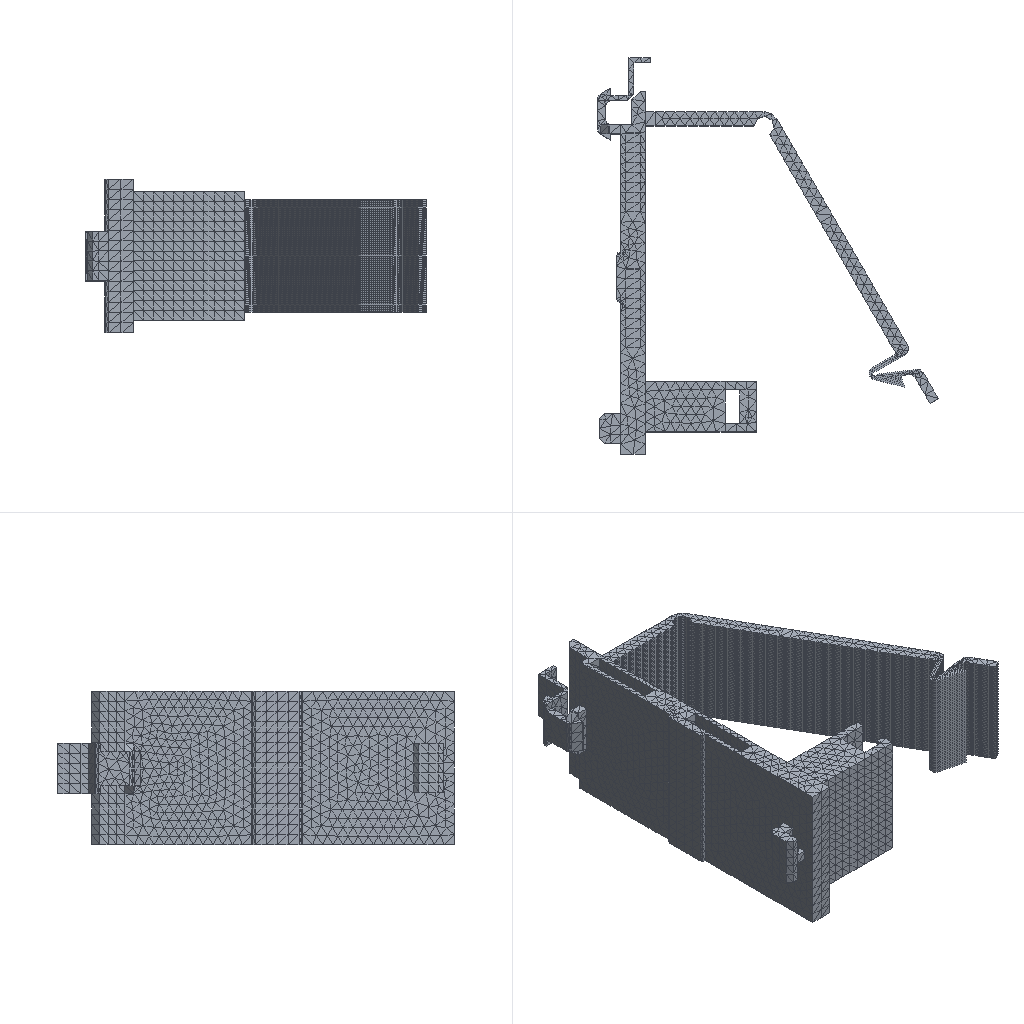Simulation study | abaqus
Set-up summary:
category,name,step,type,value,unit,region
solver,abaqus
solver,version,,,Abaqus/Standard 2020
units,not stated in the deck,,not stated
analysis,deck,,static,static
load_step,Step-1,Step-1,static
load_step,requested,,,1
mesh,nodes,,,22075
mesh,elements,,,90547
element_type,C3D4,,solid,90547
load,load commands in deck,,count,1
bc,support commands in deck,,count,7
material,MATERIAL-1,,in results
check,setup vs results,,match,"per instance, exact: element labels, types and connectivity; labels of the nodes the elements use; coordinates of those nodes at SINGLE_PRECISION in 1 of 1 instance(s)"
Abaqus input file, long lists of numbers shortened:
*Heading
** Job name: Job-2 Model name: Model-1
** Generated by: Abaqus/CAE 2020
*Preprint, echo=NO, model=NO, history=NO, contact=NO
**
** PARTS
**
*Part, name=work
*Node
      1,   3.807,  -1.262,   3.7
      2,   3.807,  -1.262,  -1.3
** (22073 more lines like these left out)
*Element, type=C3D4
    1, 14591, 14592, 14593, 14594
    2, 14591, 14595, 14596, 14594
** (90545 more lines like these left out)
*Nset, nset=Set-1, generate
     1,  22075,      1
*Elset, elset=Set-1, generate
     1,  90547,      1
** Section: Section-1
*Solid Section, elset=Set-1, material=Material-1
,
*End Part
**
**
** ASSEMBLY
**
*Assembly, name=Assembly
**
*Instance, name=work-1, part=work
*End Instance
**
*Node
      1,   16.658,   -4.462,         1.25
*Nset, nset=Set-3, instance=work-1
   104,   105,   106,   107,   108,   109,   110,   111,   112,   113,   114,   115,   116,   117,   118,   119
   120,   121,   122,   123,   205,   206,   209,   210,   217,   218,   219,   220,   223,   224,   225,   226
** (39 more lines like these left out)
*Elset, elset=Set-3, instance=work-1
   764,  2513,  4548,  6615,  8547,  8655,  9392,  9664, 10545, 10554, 10556, 10558, 10654, 10686, 12815, 12833
 12986, 12996, 13206, 13221, 13236, 13284, 13291, 13305, 13322, 13328, 13394, 13404, 13464, 13696, 14142, 15031
** (67 more lines like these left out)
*Nset, nset=Set-5
 1,
*Nset, nset=Set-6
 1,
*Nset, nset=m_Set-4
 1,
*Elset, elset=_s_Surf-1_S3, internal, instance=work-1
  1065,  3300,  9440,  9995, 12958, 13079, 13080, 13460, 13489, 13508, 13525, 13528, 13554, 13560, 13588, 13594
 14445, 14569, 14627, 14642, 14709, 14762, 14820, 15162, 15602, 15804, 16461, 17184, 17417, 17502, 18000, 18113
** (25 more lines like these left out)
*Elset, elset=_s_Surf-1_S4, internal, instance=work-1
  6947, 12110, 15494, 16739, 18273, 18904, 19107, 19441, 19514, 19558, 19605, 19740, 19774, 19808, 19878, 19909
 20085, 20116, 20253, 20968, 22709, 22964, 23125, 23432, 23584, 23605, 23741, 23742, 24158, 27091, 28853, 29818
** (2 more lines like these left out)
*Elset, elset=_s_Surf-1_S2, internal, instance=work-1
 13451, 18900, 19170, 19176, 19242, 19571, 19647, 19726, 19743, 19765, 19805, 19862, 19891, 20231, 20471, 20554
 21449, 23038, 23278, 23984, 23988, 29549, 29842, 30438, 33077, 33421, 39209, 54948, 58478, 69951, 70831, 76509
** (1 more lines like these left out)
*Elset, elset=_s_Surf-1_S1, internal, instance=work-1
 19134, 19251, 19392, 19742, 19751, 19762, 19798, 19846, 20167, 20178, 21353, 21370, 21694, 21764, 22003, 22004
 22470, 22799, 23500, 24551, 57766, 58494, 65889, 68364, 70026, 70454
*Surface, type=ELEMENT, name=s_Surf-1
_s_Surf-1_S3, S3
_s_Surf-1_S4, S4
_s_Surf-1_S2, S2
_s_Surf-1_S1, S1
*Elset, elset=_s_Surf-2_S4, internal, instance=work-1
  1164,  2199,  2690,  2870,  5811,  7944,  8257, 14253, 15244, 15617, 18853, 18854, 18866, 19575, 20898, 22227
 25708, 26415, 26669, 30098, 34360, 34378, 34963, 38395, 39354, 39389, 39423, 40444, 44348, 49840, 49921, 49978
** (5 more lines like these left out)
*Elset, elset=_s_Surf-2_S3, internal, instance=work-1
  6874, 12126, 12932, 13529, 14256, 14836, 15100, 15487, 15540, 15634, 16632, 17397, 18548, 18641, 18714, 18830
 19147, 19183, 19598, 19628, 19654, 19686, 19737, 19806, 19872, 19880, 20125, 21047, 21733, 21860, 22063, 22346
** (10 more lines like these left out)
*Elset, elset=_s_Surf-2_S1, internal, instance=work-1
 14248, 21140, 23265, 52910, 55080, 56694, 58541, 63758, 66566, 66615, 76146, 78774, 81565
*Elset, elset=_s_Surf-2_S2, internal, instance=work-1
 14684, 14796, 14845, 18949, 21197, 23723, 46722, 49241, 53451, 53829, 53860, 54862, 57325, 58957, 59065, 59920
 64158, 64175, 64252, 64405, 64463, 65348, 66297, 66598, 66650, 66991, 67034
*Surface, type=ELEMENT, name=s_Surf-2
_s_Surf-2_S4, S4
_s_Surf-2_S3, S3
_s_Surf-2_S2, S2
_s_Surf-2_S1, S1
*Elset, elset=_s_Surf-3_S4, internal, instance=work-1
   404,  1164,  1394,  1967,  2199,  2622,  2690,  2870,  3029,  3371,  3477,  3657,  5811,  6405,  6676,  7454
  7944,  8257, 11476, 14018, 14253, 14320, 15244, 15617, 17242, 18853, 18854, 18866, 18868, 19575, 19757, 20697
** (16 more lines like these left out)
*Elset, elset=_s_Surf-3_S3, internal, instance=work-1
   328,  1284,  2264,  2933,  3915,  6874,  7452,  7511,  9238, 11335, 11469, 11477, 11770, 12126, 12171, 12790
 12932, 12950, 12960, 12970, 13019, 13023, 13024, 13041, 13193, 13198, 13529, 13699, 13811, 13904, 13908, 13926
** (171 more lines like these left out)
*Elset, elset=_s_Surf-3_S1, internal, instance=work-1
   402,  2739,  4954,  6226, 11472, 12294, 14248, 15462, 20277, 20593, 21140, 23265, 24220, 29011, 29138, 29591
 30557, 30652, 30849, 31337, 31404, 31694, 33257, 33859, 34476, 34520, 34624, 34676, 34723, 34739, 35469, 35855
** (4 more lines like these left out)
*Elset, elset=_s_Surf-3_S2, internal, instance=work-1
  1620,  2009,  2935,  6231, 14684, 14796, 14845, 17188, 18949, 21197, 23723, 24383, 30551, 31366, 31614, 35305
 37994, 39980, 39981, 39988, 40055, 40547, 41770, 42297, 42310, 42420, 42471, 42925, 43365, 43770, 44062, 44070
** (3 more lines like these left out)
*Surface, type=ELEMENT, name=s_Surf-3
_s_Surf-3_S4, S4
_s_Surf-3_S3, S3
_s_Surf-3_S2, S2
_s_Surf-3_S1, S1
*Elset, elset=_s_Surf-4_S3, internal, instance=work-1
   328,  1284,  2264,  2933,  3915,  7452,  7511,  9238, 11335, 11469, 11477, 11770, 12171, 12790, 12950, 12960
 12970, 13019, 13023, 13024, 13041, 13193, 13198, 13699, 13811, 13904, 13908, 13926, 13943, 13948, 13953, 13961
** (159 more lines like these left out)
*Elset, elset=_s_Surf-4_S1, internal, instance=work-1
   402,  2739,  4954,  6226, 11472, 12294, 15462, 20277, 20593, 24220, 29011, 29138, 29591, 30557, 30652, 30849
 31337, 31404, 31694, 33257, 33859, 34476, 34520, 34624, 34676, 34723, 34739, 35469, 35855, 36039, 36429, 36634
** (3 more lines like these left out)
*Elset, elset=_s_Surf-4_S4, internal, instance=work-1
   404,  1394,  1967,  2622,  3029,  3371,  3477,  3657,  6405,  6676,  7454, 11476, 14018, 14320, 17242, 18868
 19757, 20697, 21384, 22882, 27591, 28591, 28728, 29631, 30272, 31136, 31264, 32150, 32937, 33001, 33241, 33489
** (9 more lines like these left out)
*Elset, elset=_s_Surf-4_S2, internal, instance=work-1
  1620,  2009,  2935,  6231, 17188, 24383, 30551, 31366, 31614, 35305, 37994, 39980, 39981, 39988, 40055, 40547
 41770, 42297, 42310, 42420, 42471, 42925, 43365, 43770, 44062, 44070, 44524, 46633, 47644, 47824, 48131, 59119
** (1 more lines like these left out)
*Surface, type=ELEMENT, name=s_Surf-4
_s_Surf-4_S3, S3
_s_Surf-4_S1, S1
_s_Surf-4_S4, S4
_s_Surf-4_S2, S2
*Elset, elset=_s_Surf-5_S4, internal, instance=work-1
   404,  1164,  1394,  1967,  2199,  2622,  2690,  2870,  3029,  3371,  3477,  3657,  5811,  6405,  6676,  7454
  7944,  8257, 11476, 14018, 14253, 14320, 15244, 15617, 17242, 18853, 18854, 18866, 18868, 19575, 19757, 20697
** (16 more lines like these left out)
*Elset, elset=_s_Surf-5_S3, internal, instance=work-1
   328,  1284,  2264,  2933,  3915,  6874,  7452,  7511,  9238, 11335, 11469, 11477, 11770, 12126, 12171, 12790
 12932, 12950, 12960, 12970, 13019, 13023, 13024, 13041, 13193, 13198, 13529, 13699, 13811, 13904, 13908, 13926
** (171 more lines like these left out)
*Elset, elset=_s_Surf-5_S1, internal, instance=work-1
   402,  2739,  4954,  6226, 11472, 12294, 14248, 15462, 20277, 20593, 21140, 23265, 24220, 29011, 29138, 29591
 30557, 30652, 30849, 31337, 31404, 31694, 33257, 33859, 34476, 34520, 34624, 34676, 34723, 34739, 35469, 35855
** (4 more lines like these left out)
*Elset, elset=_s_Surf-5_S2, internal, instance=work-1
  1620,  2009,  2935,  6231, 14684, 14796, 14845, 17188, 18949, 21197, 23723, 24383, 30551, 31366, 31614, 35305
 37994, 39980, 39981, 39988, 40055, 40547, 41770, 42297, 42310, 42420, 42471, 42925, 43365, 43770, 44062, 44070
** (3 more lines like these left out)
*Surface, type=ELEMENT, name=s_Surf-5
_s_Surf-5_S4, S4
_s_Surf-5_S3, S3
_s_Surf-5_S2, S2
_s_Surf-5_S1, S1
** Constraint: Constraint-1
*Coupling, constraint name=Constraint-1, ref node=m_Set-4, surface=s_Surf-5
*Kinematic
*Elset, elset=__Int-1_gcs0_13_S4, internal, instance=work-1
   625,  9876, 15059, 15485, 15785, 17626, 73124, 76096, 76213, 76242, 76267, 76358, 76369
*Elset, elset=__Int-1_gcs0_13_S2, internal, instance=work-1
 13309, 15064, 15224, 15574, 51366, 76132, 76152, 76294, 76297, 76337, 76370, 76381, 76382, 79776
*Elset, elset=__Int-1_gcs0_13_S1, internal, instance=work-1
 14332, 15793, 76351, 76359, 76371, 76447, 79369
*Elset, elset=__Int-1_gcs0_13_S3, internal, instance=work-1
 15224, 15574, 15785, 17626, 22158, 30188, 30196, 51368, 54831, 73286, 76082, 76132, 76166, 76242, 76275, 76292
 76294, 76301, 76313, 76315, 76336, 76338, 76389, 76473, 79370, 79776
*Surface, type=ELEMENT, name=_Int-1_gcs0_13, internal
__Int-1_gcs0_13_S4, S4
__Int-1_gcs0_13_S2, S2
__Int-1_gcs0_13_S1, S1
__Int-1_gcs0_13_S3, S3
*Elset, elset=__Int-1_gcs0_31_S4, internal, instance=work-1
   264, 27917, 40028, 77407, 77893, 78753, 78805, 78914
*Elset, elset=__Int-1_gcs0_31_S2, internal, instance=work-1
   522, 78714, 78771, 78855
*Elset, elset=__Int-1_gcs0_31_S3, internal, instance=work-1
 13304, 17602, 27908, 27924, 36808, 42413, 46779, 47763, 55089, 55101, 73750, 73804, 75296, 77222, 77407, 77602
 77978, 78663, 78714, 78753, 78755, 78757, 78783, 78794, 78795, 78806, 78819, 78825, 78830, 78841, 78864, 78882
** (1 more lines like these left out)
*Elset, elset=__Int-1_gcs0_31_S1, internal, instance=work-1
 22142, 73053, 73804, 78841, 78842, 78854, 78926
*Surface, type=ELEMENT, name=_Int-1_gcs0_31, internal
__Int-1_gcs0_31_S4, S4
__Int-1_gcs0_31_S2, S2
__Int-1_gcs0_31_S3, S3
__Int-1_gcs0_31_S1, S1
*Elset, elset=__Int-1_gcs0_48_S4, internal, instance=work-1
  5307,  6871, 17964
*Elset, elset=__Int-1_gcs0_48_S2, internal, instance=work-1
 5412,
*Elset, elset=__Int-1_gcs0_48_S3, internal, instance=work-1
 16681, 16696, 17965, 17990, 17993, 20741, 20748, 46122
*Surface, type=ELEMENT, name=_Int-1_gcs0_48, internal
__Int-1_gcs0_48_S4, S4
__Int-1_gcs0_48_S2, S2
__Int-1_gcs0_48_S3, S3
*Elset, elset=__Int-1_gcs0_51_S3, internal, instance=work-1
 16470, 16660
*Surface, type=ELEMENT, name=_Int-1_gcs0_51, internal
__Int-1_gcs0_51_S3, S3
*Elset, elset=__Int-1_gcs0_60_S3, internal, instance=work-1
 17957, 23130
*Surface, type=ELEMENT, name=_Int-1_gcs0_60, internal
__Int-1_gcs0_60_S3, S3
*Elset, elset=__Int-1_gcs0_65_S4, internal, instance=work-1
 16377, 17008, 17019, 79449
*Elset, elset=__Int-1_gcs0_65_S2, internal, instance=work-1
 16449, 79453
*Elset, elset=__Int-1_gcs0_65_S3, internal, instance=work-1
 16684, 16710, 16948, 17001, 17005, 79459
*Surface, type=ELEMENT, name=_Int-1_gcs0_65, internal
__Int-1_gcs0_65_S4, S4
__Int-1_gcs0_65_S2, S2
__Int-1_gcs0_65_S3, S3
*Elset, elset=__Int-1_gcs0_68_S3, internal, instance=work-1
 16669, 16702, 16787, 16792, 16813, 16816, 20746, 25844, 25858, 68939, 90333
*Elset, elset=__Int-1_gcs0_68_S2, internal, instance=work-1
 16782,
*Surface, type=ELEMENT, name=_Int-1_gcs0_68, internal
__Int-1_gcs0_68_S3, S3
__Int-1_gcs0_68_S2, S2
*Elset, elset=__Int-1_gcs0_71_S3, internal, instance=work-1
 16293, 16364, 16372, 16380, 16404, 16412, 16439, 16443, 16453, 16459, 16481, 16485, 16560, 16880, 16945, 34472
 79452, 90309, 90310, 90312
*Surface, type=ELEMENT, name=_Int-1_gcs0_71, internal
__Int-1_gcs0_71_S3, S3
*Elset, elset=__Int-1_gcs0_77_S4, internal, instance=work-1
 13427, 15299, 15734, 15737, 15844, 16178, 16538, 66174
*Elset, elset=__Int-1_gcs0_77_S2, internal, instance=work-1
 15721, 16168
*Elset, elset=__Int-1_gcs0_77_S1, internal, instance=work-1
 15750, 16081, 30318
*Elset, elset=__Int-1_gcs0_77_S3, internal, instance=work-1
 15876, 16119, 16180, 16181, 16528, 16549, 61831
*Surface, type=ELEMENT, name=_Int-1_gcs0_77, internal
__Int-1_gcs0_77_S4, S4
__Int-1_gcs0_77_S2, S2
__Int-1_gcs0_77_S1, S1
__Int-1_gcs0_77_S3, S3
*Elset, elset=__Int-1_gcs0_105_S3, internal, instance=work-1
 12941, 12951, 13242, 13676, 13762, 13778, 14410, 14573, 14580, 14583, 14812, 15607, 17445, 18443, 19934, 19937
 20180, 20417, 20495, 20577, 20897, 20911, 21137, 21220, 21222, 21279, 21292, 21539, 21611, 21849, 21929, 22085
** (17 more lines like these left out)
*Elset, elset=__Int-1_gcs0_105_S1, internal, instance=work-1
 20335, 24373, 24644, 25023, 25054, 25095, 25100, 25404, 25407, 25877, 30499, 31827, 40049, 45088, 45102, 50731
 55417, 55818, 58462, 64160, 70267
*Elset, elset=__Int-1_gcs0_105_S4, internal, instance=work-1
 22808, 24588, 24874, 24895, 54570, 55237, 55780, 57816, 59475, 62871, 64537
*Surface, type=ELEMENT, name=_Int-1_gcs0_105, internal
__Int-1_gcs0_105_S3, S3
__Int-1_gcs0_105_S1, S1
__Int-1_gcs0_105_S4, S4
*Elset, elset=__Int-1_gcs0_109_S3, internal, instance=work-1
  1458,  3403,  3822,  3824, 11598, 12627, 12713, 13054, 13567, 13989, 18306, 18317, 18402, 18507, 18832, 18947
 19103, 19234, 19267, 22368, 22434, 22518, 24892, 24952, 24971, 28615, 31234, 37971, 38141, 42138, 45090, 45149
** (9 more lines like these left out)
*Elset, elset=__Int-1_gcs0_109_S1, internal, instance=work-1
  3401, 11595, 18579, 23915, 31120, 31236, 33437, 55446, 78327
*Elset, elset=__Int-1_gcs0_109_S2, internal, instance=work-1
  4990, 18530, 41570, 46175, 55453, 59818, 61190, 64445, 64534, 65243, 66318, 67075, 67964, 68148, 68225, 68313
 68359, 68459, 73859, 73889, 73905, 74119, 76550
*Elset, elset=__Int-1_gcs0_109_S4, internal, instance=work-1
 12215, 43493, 53176, 55445, 59576, 64088, 64486, 65353, 68342, 68439, 74154, 74224, 74506
*Surface, type=ELEMENT, name=_Int-1_gcs0_109, internal
__Int-1_gcs0_109_S3, S3
__Int-1_gcs0_109_S1, S1
__Int-1_gcs0_109_S2, S2
__Int-1_gcs0_109_S4, S4
*Elset, elset=__Int-1_gcs0_111_S3, internal, instance=work-1
  2024,  4240,  9647, 11771, 11966, 13060, 14884, 18504, 18937, 19063, 19308, 19373, 19466, 19630, 19640, 21371
 21453, 21605, 25845, 27458, 27756, 33141, 33960, 35297, 38821, 38976, 39918, 40366, 40446, 40980, 45453, 48255
** (9 more lines like these left out)
*Elset, elset=__Int-1_gcs0_111_S4, internal, instance=work-1
  4139, 18505, 46522, 47587, 54504, 55629, 57193, 57573, 57665, 58132, 63781, 65107, 66151, 66180, 67501, 67536
 67546, 67759, 67779, 68210, 68488, 74485, 78277, 82041, 84962
*Elset, elset=__Int-1_gcs0_111_S2, internal, instance=work-1
 12270, 16930, 56881, 58799, 62596, 67544
*Elset, elset=__Int-1_gcs0_111_S1, internal, instance=work-1
 21538, 26913, 27460, 30568, 30679, 35475, 47877, 55214, 55219, 55295, 57195, 57781, 58266, 68956, 80440, 81355
 89091,
*Surface, type=ELEMENT, name=_Int-1_gcs0_111, internal
__Int-1_gcs0_111_S3, S3
__Int-1_gcs0_111_S4, S4
__Int-1_gcs0_111_S2, S2
__Int-1_gcs0_111_S1, S1
*Elset, elset=__Int-1_gcs0_115_S4, internal, instance=work-1
   627,  1957,  6048, 10321, 21535, 24498, 27524, 48409, 58082, 63898, 63939, 64030, 66730, 89904
*Elset, elset=__Int-1_gcs0_115_S3, internal, instance=work-1
  6050,  6705,  7647,  8021,  9513, 13133, 13134, 13167, 13456, 13541, 14851, 16510, 18693, 18821, 18891, 19197
 19243, 19398, 19504, 19626, 19856, 19879, 20469, 21885, 24066, 24221, 26719, 26727, 28154, 29397, 30879, 37876
** (10 more lines like these left out)
*Elset, elset=__Int-1_gcs0_115_S1, internal, instance=work-1
  6052, 27405, 27825, 48173, 50606, 51573, 66818, 67713, 75175, 75221, 84974
*Elset, elset=__Int-1_gcs0_115_S2, internal, instance=work-1
 19676, 63524, 64028, 64101
*Surface, type=ELEMENT, name=_Int-1_gcs0_115, internal
__Int-1_gcs0_115_S4, S4
__Int-1_gcs0_115_S3, S3
__Int-1_gcs0_115_S2, S2
__Int-1_gcs0_115_S1, S1
*Elset, elset=__Int-1_gcs0_117_S3, internal, instance=work-1
 10776, 13083, 13088, 13659, 13660, 13693, 14507, 14606, 15583, 16075, 17693, 18993, 19409, 19512, 19516, 19530
 19931, 20182, 20357, 20585, 20662, 20984, 21058, 21060, 21144, 21153, 21381, 21714, 22021, 22094, 22557, 22570
** (37 more lines like these left out)
*Elset, elset=__Int-1_gcs0_117_S4, internal, instance=work-1
 11527, 15004, 26293, 40499, 44545, 55292, 56057, 56199, 59016, 59020, 69704, 80517, 81548, 90315
*Elset, elset=__Int-1_gcs0_117_S2, internal, instance=work-1
 19500, 24321, 24419, 24628, 25288, 25718, 26691, 40563, 47016, 51711, 55519, 55551, 55868, 55985, 56207, 59079
 60555, 72504, 73599, 87102, 89637
*Elset, elset=__Int-1_gcs0_117_S1, internal, instance=work-1
 28984, 31149, 44732, 47978, 59077, 63191, 63706, 66257, 67328, 72568
*Surface, type=ELEMENT, name=_Int-1_gcs0_117, internal
__Int-1_gcs0_117_S3, S3
__Int-1_gcs0_117_S4, S4
__Int-1_gcs0_117_S2, S2
__Int-1_gcs0_117_S1, S1
*Elset, elset=__Int-1_gcs0_119_S1, internal, instance=work-1
   710,  3316,  5613,  6938, 12251, 27224, 48569, 74586, 74601
*Elset, elset=__Int-1_gcs0_119_S4, internal, instance=work-1
   712,  2002,  3750,  8757,  8758,  9017, 14438, 28462, 45847, 48245, 48316, 48529, 48699, 48720, 49821, 51891
 63198, 70807
*Elset, elset=__Int-1_gcs0_119_S3, internal, instance=work-1
  3881,  6935, 10823, 13802, 14429, 14440, 14545, 14549, 14624, 14639, 19407, 19666, 27639, 27662, 27829, 27951
 28461, 28463, 28828, 29140, 29331, 29586, 29747, 30139, 30703, 30920, 31049, 31139, 31142, 31183, 31396, 31647
** (10 more lines like these left out)
*Elset, elset=__Int-1_gcs0_119_S2, internal, instance=work-1
 19138, 48745, 49102
*Surface, type=ELEMENT, name=_Int-1_gcs0_119, internal
__Int-1_gcs0_119_S1, S1
__Int-1_gcs0_119_S4, S4
__Int-1_gcs0_119_S2, S2
__Int-1_gcs0_119_S3, S3
*Elset, elset=__Int-1_gcs0_121_S4, internal, instance=work-1
  6222, 13795, 15184, 21770, 24333, 25228, 35192, 38414, 38564, 38749, 38781, 38833, 38889, 38919, 38937, 38947
 38972, 39207, 39329, 39330, 39332, 39345, 39347, 39419, 39570, 39704, 39837, 43386, 53186, 58487, 63307, 67444
** (2 more lines like these left out)
*Elset, elset=__Int-1_gcs0_121_S3, internal, instance=work-1
  8096, 14934, 18884, 21030, 21829, 24503, 27598, 38525, 38536, 38629, 38815, 38948, 39058, 39154, 39241, 39304
 39305, 39382, 39472, 39512, 39668, 39703, 39800, 44181, 55567, 66207, 67133, 68522, 68756, 68823, 68862, 68884
** (2 more lines like these left out)
*Elset, elset=__Int-1_gcs0_121_S1, internal, instance=work-1
 11802, 12611, 21464, 21686, 21695, 21830, 24617, 38140, 38336, 39091, 39213, 39298, 39355, 39384, 39488, 39661
 39684, 39733, 39808, 39952, 58293, 58298, 58327, 63285, 67885, 68474, 68725, 68913, 68971, 69365, 69518, 69713
** (1 more lines like these left out)
*Elset, elset=__Int-1_gcs0_121_S2, internal, instance=work-1
 12980, 14914, 14917, 19711, 21808, 24668, 24755, 25004, 25112, 25192, 33856, 34173, 35242, 38330, 38552, 38862
 38864, 38932, 39012, 39060, 39177, 39207, 39250, 39447, 39635, 39779, 39913, 48665, 58013, 58234, 58490, 63312
** (2 more lines like these left out)
*Surface, type=ELEMENT, name=_Int-1_gcs0_121, internal
__Int-1_gcs0_121_S4, S4
__Int-1_gcs0_121_S3, S3
__Int-1_gcs0_121_S2, S2
__Int-1_gcs0_121_S1, S1
*Elset, elset=__Int-1_gcs0_125_S3, internal, instance=work-1
  5835,  6664,  7393,  9693, 11200, 13656, 13682, 14155, 14156, 14494, 14526, 15183, 15438, 16099, 17059, 17504
 17927, 17959, 18846, 19220, 19357, 19393, 19416, 19493, 20411, 20740, 20818, 21970, 22010, 22400, 22887, 23460
** (31 more lines like these left out)
*Elset, elset=__Int-1_gcs0_125_S1, internal, instance=work-1
 23464, 24582, 46103, 54630
*Elset, elset=__Int-1_gcs0_125_S4, internal, instance=work-1
 24748, 25775, 26259, 26321, 27003, 28774, 52803, 53967, 54794, 55443, 58960, 71225, 78103, 89445, 89450, 89490
*Elset, elset=__Int-1_gcs0_125_S2, internal, instance=work-1
 25527, 26059, 26197, 26711, 26918, 34161, 43896, 49282, 73576, 73696, 77381, 89190, 89644
*Surface, type=ELEMENT, name=_Int-1_gcs0_125, internal
__Int-1_gcs0_125_S3, S3
__Int-1_gcs0_125_S1, S1
__Int-1_gcs0_125_S4, S4
__Int-1_gcs0_125_S2, S2
*Elset, elset=__Int-1_gcs0_128_S4, internal, instance=work-1
  2297,  5848, 13625, 13768, 13966, 14906, 15383, 15718, 16599, 16892, 18777, 25186, 27689, 31347, 38102, 38599
 38830, 38912, 39311, 39393, 39538, 39568, 39749, 39910, 39954, 41421, 41836, 46963, 55002, 55041, 65076, 67434
** (3 more lines like these left out)
*Elset, elset=__Int-1_gcs0_128_S2, internal, instance=work-1
  3735,  4955,  6388, 18670, 21054, 25645, 27583, 32094, 38019, 38921, 39212, 39636, 39682, 40417, 42279, 55605
 64756, 67059, 68028, 68722, 68724, 68937, 68978, 69235, 69344, 69369, 69372, 69400, 69580, 69741, 69786, 69946
** (1 more lines like these left out)
*Elset, elset=__Int-1_gcs0_128_S3, internal, instance=work-1
  8880, 11490, 12367, 12992, 13002, 13990, 14048, 14051, 14057, 14072, 14078, 14904, 14927, 15229, 15253, 15861
 15919, 16036, 17517, 18622, 20810, 20956, 21685, 21702, 21741, 22609, 24823, 24960, 25051, 27590, 27593, 28384
** (24 more lines like these left out)
*Elset, elset=__Int-1_gcs0_128_S1, internal, instance=work-1
 13597, 14284, 14334, 14928, 14930, 15101, 24499, 38433, 39179, 39312, 39428, 39592, 41834, 45694, 49596, 58306
 58460, 58538, 58599, 67973, 68175, 68672, 68904, 68965, 69199, 69279, 69579, 69920, 70472, 79641, 87619, 88295
** (1 more lines like these left out)
*Surface, type=ELEMENT, name=_Int-1_gcs0_128, internal
__Int-1_gcs0_128_S4, S4
__Int-1_gcs0_128_S2, S2
__Int-1_gcs0_128_S3, S3
__Int-1_gcs0_128_S1, S1
*End Assembly
**
** MATERIALS
**
*Material, name=Material-1
*Density
 1.15e-09,
*Elastic
1060., 0.35
**
** INTERACTION PROPERTIES
**
*Surface Interaction, name=IntProp-1
1.,
*Friction, slip tolerance=0.005
 0.4,
*Surface Behavior, pressure-overclosure=HARD
**
** INTERACTIONS
**
** Interaction: Int-1
*Contact
*Contact Inclusions, ALL EXTERIOR
*Contact Property Assignment
 ,  , IntProp-1
*Surface Property Assignment, property=GEOMETRIC CORRECTION
_Int-1_gcs0_13, Circumferential, 2.457, -21.462, -26.165,  2.457, -21.462, -27.165
_Int-1_gcs0_31, Circumferential, 2.457, -17.162, 28.665,  2.457, -17.162, 29.665
_Int-1_gcs0_48, Circumferential, 1.507, -3.762, 28.665,  1.507, -3.762, 29.665
_Int-1_gcs0_51, Circumferential, 1.39, 53.489, 3.5,  1.39, 54.489, 3.5
_Int-1_gcs0_60, Circumferential, 1.39, -75.198, -1.1,  1.39, -76.198, -1.1
_Int-1_gcs0_65, Circumferential, 1.507, -2.362, -26.165,  1.507, -2.362, -27.165
_Int-1_gcs0_68, Circumferential, 0.707, -4.758, -26.165,  0.707, -4.758, -27.165
_Int-1_gcs0_71, Circumferential, 0.707, -1.644, 28.665,  0.707, -1.644, 29.665
_Int-1_gcs0_77, Circumferential, 3.007, -1.062, 3.7,  3.007, -1.062, 4.7
_Int-1_gcs0_105, Circumferential, 27.676, -28.847, -26.165,  27.676, -28.847, -27.165
_Int-1_gcs0_109, Circumferential, 30.426, -29.196, 6.35,  30.426, -29.196, 7.35
_Int-1_gcs0_111, Circumferential, 31.067, -29.52, 6.35,  31.067, -29.52, 5.35
_Int-1_gcs0_115, Circumferential, 31.874, -29.018, 6.35,  31.874, -29.018, 7.35
_Int-1_gcs0_117, Circumferential, 27.64, -28.829, 6.35,  27.64, -28.829, 7.35
_Int-1_gcs0_119, Circumferential, 30.376, -26.423, -26.165,  30.376, -26.423, -27.165
_Int-1_gcs0_121, Circumferential, 16.657, -4.462, 6.35,  16.657, -4.462, 5.35
_Int-1_gcs0_125, Circumferential, 27.651, -28.804, -26.165,  27.651, -28.804, -27.165
_Int-1_gcs0_128, Circumferential, 16.665, -4.412, 4.3,  16.665, -4.412, 5.3
** ----------------------------------------------------------------
**
** STEP: Step-1
**
*Step, name=Step-1, nlgeom=YES, inc=10000
*Static, stabilize=0.0002, allsdtol=0.05, continue=NO
0.01, 1., 1e-05, 1.
**
** BOUNDARY CONDITIONS
**
** Name: fixed Type: 对称/反对称/完全固定
*Boundary
Set-3, ENCASTRE
** Name: weiyi Type: Displacement/Rotation angle
*Boundary
Set-6, 1, 1
Set-6, 2, 2
Set-6, 3, 3
Set-6, 4, 4
Set-6, 5, 5
Set-6, 6, 6, -31.7
**
** OUTPUT REQUESTS
**
*Restart, write, number interval=1, time marks=NO
**
** FIELD OUTPUT: F-Output-1
**
*Output, field
*Node Output
RF, U, V
*Element Output, directions=YES
E, LE, MISES, PE, PEEQ, S
*Contact Output
CDISP, CSTRESS
**
** HISTORY OUTPUT: H-Output-1
**
*Output, history, number interval=1000, time marks=NO
*Node Output, nset=m_Set-4
RF1, RF2, RF3, RM1, RM2, RM3, U1, U2
U3, UR1, UR2, UR3
*End Step
Results summary:
result,step,,partial,increments=29 time=0.01655/1.0
result,analysis,,,static
result,last_loadstep,,,1
result,primary field,,,U
result,reaction total,,FX,-0.2388,model units
result,reaction total,,FY,-0.2819,model units
result,reaction total,,FZ,-0.00487,model units